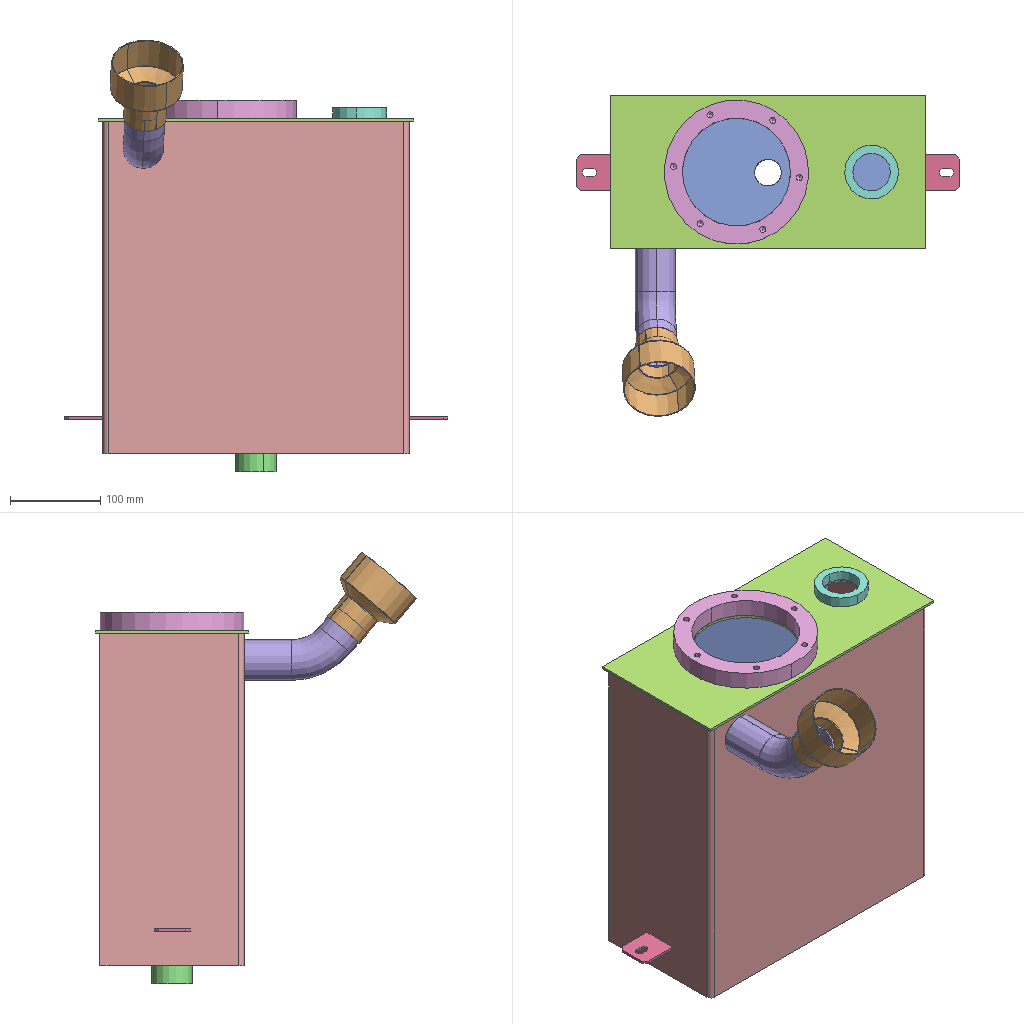Assembly | SolidWorks | 9 different items | 11 placed | box 426 x 356 x 479 mm
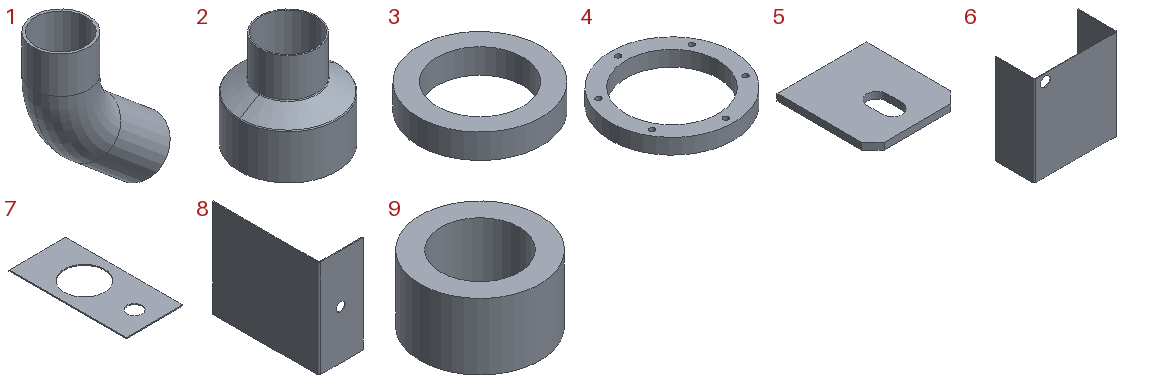Parts list (item | quantity | size | volume | features):
1 | x1 | 99.465 x 45 x 128.591 mm | 36956 mm3 | features Shell 1, Sweep 1
2 | x1 | 80 x 80 x 79 mm | 17561 mm3 | features 3DProfileFeature 2, ICE 2, Blend 1, Fillet 1, Shell 1
3 | x1 | 60 x 60 x 12 mm | 17462 mm3 | features Extrusion 1
4 | x1 | 160 x 160 x 20 mm | 171859 mm3 | features 3DProfileFeature 1, Extrusion 1, HoleWzd 1
5 | x2 | 40 x 43 x 3 mm | 4705 mm3 | features Extrusion 1
6 | x1 | 340 x 160 x 369 mm | 715620 mm3 | features Cut 2, FlatPattern 1, SMBaseFlange 1, SheetMetal 1
7 | x1 | 170 x 350 x 3 mm | 139800 mm3 | features Extrusion 1
8 | x1 | 152 x 364 x 334 mm | 509961 mm3 | features Cut 1, FlatPattern 1, ICE 1, SMBaseFlange 1, SheetMetal 1
9 | x2 | 45 x 45 x 25 mm | 22673 mm3 | features Extrusion 1
Mates (type | each side: item.copy, entity, surface, feature):
Coincident | 6.1 face plane Base-Flange1 | 8.1 face plane Base-Flange1 | 2 times
DistanceDim | 8.1 face plane Base-Flange1 | 6.1 face plane Base-Flange1
Coincident | 6.1 face plane Base-Flange1 | 7.1 face plane Boss-Extrude1
DistanceDim | 7.1 face plane Boss-Extrude1 | 6.1 face plane Base-Flange1 | 2 times
Concentric | 7.1 edge | 4.1 edge
Coincident | 7.1 face plane Boss-Extrude1 | 4.1 face plane Boss-Extrude1
Concentric | 7.1 edge | 3.1 edge
Coincident | 7.1 face plane Boss-Extrude1 | 3.1 face plane Boss-Extrude1
Coincident | 6.1 face plane Base-Flange1 | 1.1 face plane Sweep1
Concentric | 2.1 edge | 1.1 edge
Concentric | 6.1 edge | 1.1 edge
Concentric | 8.1 edge | 9.1 edge
Coincident | 8.1 face plane Base-Flange1 | 9.1 face plane Boss-Extrude1
Coincident | 6.1 face plane Base-Flange1 | 5.1 face plane Boss-Extrude1
DistanceDim | 5.1 face plane Boss-Extrude1 | 6.1 face plane Base-Flange1 | 2 times
Coincident | 5.1 face plane Boss-Extrude1 | 5.2 face plane Boss-Extrude1 | 2 times
Coincident | 6.1 face plane Base-Flange1 | 5.2 face plane Boss-Extrude1